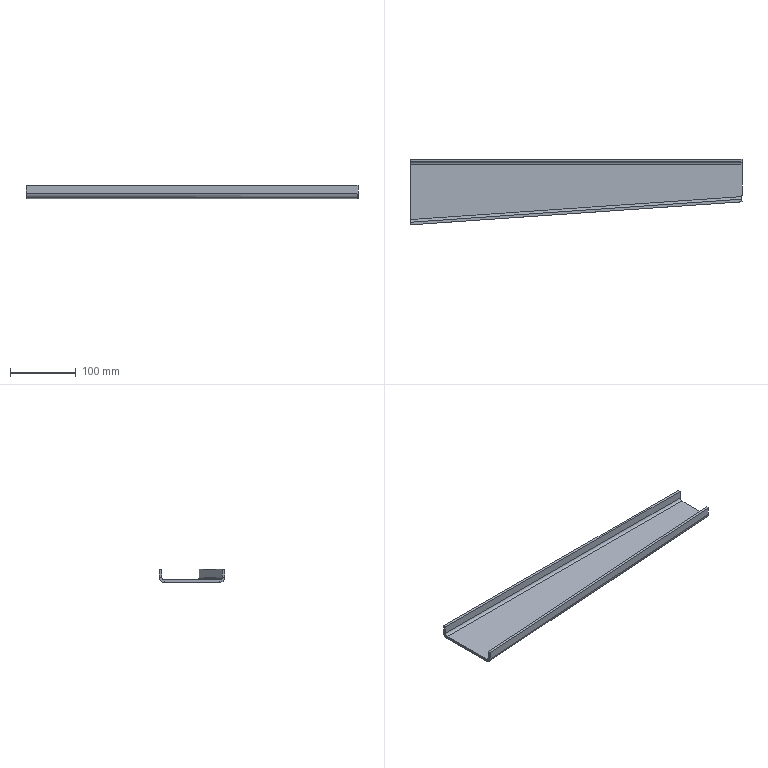Part | STEP file | 01-Bent plate 11 | 1 solid | 24 faces | box 505.277 x 100 x 20 mm | volume 220935 mm3 | plane 19 | cylinder 4 | spline 1 | commonest cylinder face diameters 8 x2 16 x2